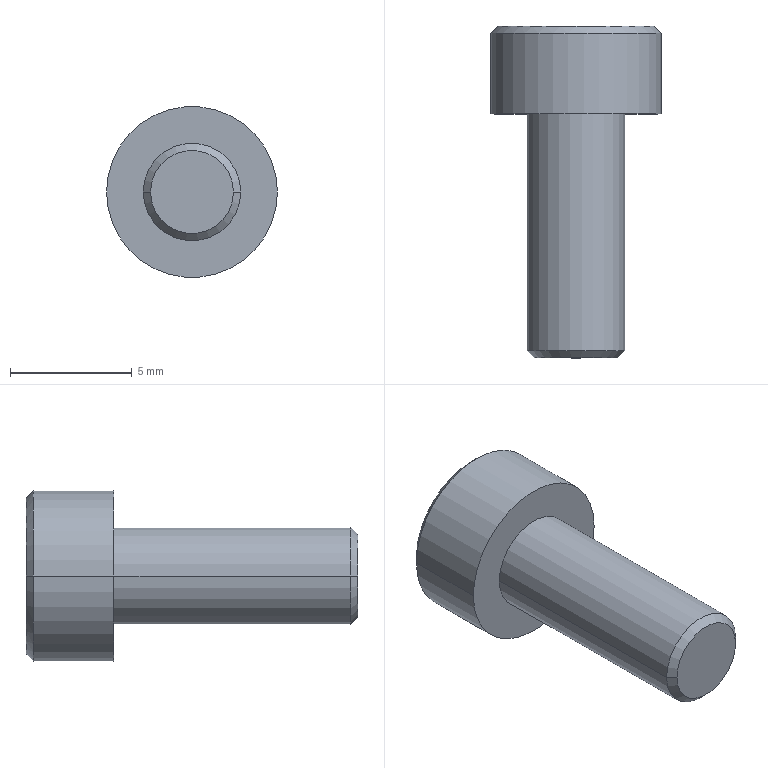Part | NX | 1 solid | 56 faces | box 7 x 13.6 x 7 mm | volume 246.76 mm3 | plane 44 | cone 6 | cylinder 6 | commonest cylinder face diameters 3 x2 4 x2 7 x2
STEP:
#1=CARTESIAN_POINT('',(1.7,-10.,0.));
#2=VERTEX_POINT('',#1);
#3=CARTESIAN_POINT('',(-1.7,-10.,0.));
#4=VERTEX_POINT('',#3);
#5=CARTESIAN_POINT('',(0.,-10.,0.));
#6=DIRECTION('',(0.,1.,0.));
#7=DIRECTION('',(-1.,0.,0.));
#8=AXIS2_PLACEMENT_3D('',#5,#6,#7);
#9=CIRCLE('',#8,1.7);
#10=EDGE_CURVE('',#2,#4,#9,.T.);
#11=ORIENTED_EDGE('',*,*,#10,.F.);
#12=CARTESIAN_POINT('',(0.,-10.,0.));
#13=DIRECTION('',(0.,1.,0.));
#14=DIRECTION('',(-1.,0.,0.));
#15=AXIS2_PLACEMENT_3D('',#12,#13,#14);
#16=CIRCLE('',#15,1.7);
#17=EDGE_CURVE('',#4,#2,#16,.T.);
#18=ORIENTED_EDGE('',*,*,#17,.F.);
#19=EDGE_LOOP('',(#11,#18));
#20=FACE_BOUND('',#19,.T.);
#21=CARTESIAN_POINT('',(0.,-10.,0.));
#22=DIRECTION('',(0.,-1.,0.));
#23=DIRECTION('',(0.,0.,-1.));
#24=AXIS2_PLACEMENT_3D('',#21,#22,#23);
#25=PLANE('',#24);
#26=ADVANCED_FACE('',(#20),#25,.T.);
#27=ORIENTED_EDGE('',*,*,#10,.T.);
#28=CARTESIAN_POINT('',(-2.,-9.7,0.));
#29=VERTEX_POINT('',#28);
#30=CARTESIAN_POINT('',(-1.85,-9.85,0.));
#31=DIRECTION('',(-0.7071,0.7071,0.));
#32=VECTOR('',#31,1000.);
#33=LINE('',#30,#32);
#34=EDGE_CURVE('',#4,#29,#33,.T.);
#35=ORIENTED_EDGE('',*,*,#34,.T.);
#36=CARTESIAN_POINT('',(2.,-9.7,0.));
#37=VERTEX_POINT('',#36);
#38=CARTESIAN_POINT('',(0.,-9.7,0.));
#39=DIRECTION('',(0.,1.,0.));
#40=DIRECTION('',(-1.,0.,0.));
#41=AXIS2_PLACEMENT_3D('',#38,#39,#40);
#42=CIRCLE('',#41,2.);
#43=EDGE_CURVE('',#37,#29,#42,.T.);
#44=ORIENTED_EDGE('',*,*,#43,.F.);
#45=CARTESIAN_POINT('',(1.85,-9.85,0.));
#46=DIRECTION('',(0.7071,0.7071,0.));
#47=VECTOR('',#46,1000.);
#48=LINE('',#45,#47);
#49=EDGE_CURVE('',#2,#37,#48,.T.);
#50=ORIENTED_EDGE('',*,*,#49,.F.);
#51=EDGE_LOOP('',(#27,#35,#44,#50));
#52=FACE_BOUND('',#51,.T.);
#53=CARTESIAN_POINT('',(0.,-9.85,0.));
#54=DIRECTION('',(0.,1.,0.));
#55=DIRECTION('',(1.,0.,0.));
#56=AXIS2_PLACEMENT_3D('',#53,#54,#55);
#57=CONICAL_SURFACE('',#56,1.85,0.7854);
#58=ADVANCED_FACE('',(#52),#57,.T.);
#59=ORIENTED_EDGE('',*,*,#43,.T.);
#60=CARTESIAN_POINT('',(-2.,0.,0.));
#61=VERTEX_POINT('',#60);
#62=CARTESIAN_POINT('',(-2.,4.28,0.));
#63=DIRECTION('',(0.,-1.,0.));
#64=VECTOR('',#63,1000.);
#65=LINE('',#62,#64);
#66=EDGE_CURVE('',#29,#61,#65,.F.);
#67=ORIENTED_EDGE('',*,*,#66,.T.);
#68=CARTESIAN_POINT('',(2.,0.,0.));
#69=VERTEX_POINT('',#68);
#70=CARTESIAN_POINT('',(0.,0.,0.));
#71=DIRECTION('',(0.,-1.,0.));
#72=DIRECTION('',(-1.,0.,0.));
#73=AXIS2_PLACEMENT_3D('',#70,#71,#72);
#74=CIRCLE('',#73,2.);
#75=EDGE_CURVE('',#61,#69,#74,.T.);
#76=ORIENTED_EDGE('',*,*,#75,.T.);
#77=CARTESIAN_POINT('',(2.,4.28,0.));
#78=DIRECTION('',(0.,-1.,0.));
#79=VECTOR('',#78,1000.);
#80=LINE('',#77,#79);
#81=EDGE_CURVE('',#37,#69,#80,.F.);
#82=ORIENTED_EDGE('',*,*,#81,.F.);
#83=EDGE_LOOP('',(#59,#67,#76,#82));
#84=FACE_BOUND('',#83,.T.);
#85=CARTESIAN_POINT('',(0.,4.28,0.));
#86=DIRECTION('',(0.,-1.,0.));
#87=DIRECTION('',(-1.,0.,0.));
#88=AXIS2_PLACEMENT_3D('',#85,#86,#87);
#89=CYLINDRICAL_SURFACE('',#88,2.);
#90=ADVANCED_FACE('',(#84),#89,.T.);
#91=CARTESIAN_POINT('',(0.1875,3.6,1.945));
#92=VERTEX_POINT('',#91);
#93=CARTESIAN_POINT('',(0.4,3.6,1.702));
#94=VERTEX_POINT('',#93);
#95=CARTESIAN_POINT('',(0.1875,3.6,1.945));
#96=DIRECTION('',(0.659,0.,-0.7522));
#97=VECTOR('',#96,1000.);
#98=LINE('',#95,#97);
#99=EDGE_CURVE('',#92,#94,#98,.T.);
#100=ORIENTED_EDGE('',*,*,#99,.T.);
#101=CARTESIAN_POINT('',(0.4,3.55,1.702));
#102=VERTEX_POINT('',#101);
#103=CARTESIAN_POINT('',(0.4,3.55,1.702));
#104=DIRECTION('',(0.,1.,0.));
#105=VECTOR('',#104,1000.);
#106=LINE('',#103,#105);
#107=EDGE_CURVE('',#102,#94,#106,.T.);
#108=ORIENTED_EDGE('',*,*,#107,.F.);
#109=CARTESIAN_POINT('',(0.1875,3.55,1.945));
#110=VERTEX_POINT('',#109);
#111=CARTESIAN_POINT('',(0.4,3.55,1.702));
#112=DIRECTION('',(-0.659,0.,0.7522));
#113=VECTOR('',#112,1000.);
#114=LINE('',#111,#113);
#115=EDGE_CURVE('',#102,#110,#114,.T.);
#116=ORIENTED_EDGE('',*,*,#115,.T.);
#117=CARTESIAN_POINT('',(0.1875,3.55,1.945));
#118=DIRECTION('',(0.,1.,0.));
#119=VECTOR('',#118,1000.);
#120=LINE('',#117,#119);
#121=EDGE_CURVE('',#110,#92,#120,.T.);
#122=ORIENTED_EDGE('',*,*,#121,.T.);
#123=EDGE_LOOP('',(#100,#108,#116,#122));
#124=FACE_BOUND('',#123,.T.);
#125=CARTESIAN_POINT('',(0.1875,3.6,1.945));
#126=DIRECTION('',(0.7522,0.,0.659));
#127=DIRECTION('',(0.,-1.,0.));
#128=AXIS2_PLACEMENT_3D('',#125,#126,#127);
#129=PLANE('',#128);
#130=ADVANCED_FACE('',(#124),#129,.F.);
#131=CARTESIAN_POINT('',(0.1,3.55,1.945));
#132=VERTEX_POINT('',#131);
#133=CARTESIAN_POINT('',(0.4,3.55,1.6));
#134=VERTEX_POINT('',#133);
#135=CARTESIAN_POINT('',(0.1,3.55,1.945));
#136=DIRECTION('',(0.6565,0.,-0.7543));
#137=VECTOR('',#136,1000.);
#138=LINE('',#135,#137);
#139=EDGE_CURVE('',#132,#134,#138,.T.);
#140=ORIENTED_EDGE('',*,*,#139,.F.);
#141=CARTESIAN_POINT('',(0.1,3.55,2.021));
#142=VERTEX_POINT('',#141);
#143=CARTESIAN_POINT('',(0.1,3.55,2.021));
#144=DIRECTION('',(0.,0.,-1.));
#145=VECTOR('',#144,1000.);
#146=LINE('',#143,#145);
#147=EDGE_CURVE('',#142,#132,#146,.T.);
#148=ORIENTED_EDGE('',*,*,#147,.F.);
#149=CARTESIAN_POINT('',(0.4,3.55,2.021));
#150=VERTEX_POINT('',#149);
#151=CARTESIAN_POINT('',(0.4,3.55,2.021));
#152=DIRECTION('',(-1.,0.,0.));
#153=VECTOR('',#152,1000.);
#154=LINE('',#151,#153);
#155=EDGE_CURVE('',#150,#142,#154,.T.);
#156=ORIENTED_EDGE('',*,*,#155,.F.);
#157=CARTESIAN_POINT('',(0.4,3.55,2.2));
#158=VERTEX_POINT('',#157);
#159=CARTESIAN_POINT('',(0.4,3.55,2.2));
#160=DIRECTION('',(0.,0.,-1.));
#161=VECTOR('',#160,1000.);
#162=LINE('',#159,#161);
#163=EDGE_CURVE('',#158,#150,#162,.T.);
#164=ORIENTED_EDGE('',*,*,#163,.F.);
#165=CARTESIAN_POINT('',(0.475,3.55,2.2));
#166=VERTEX_POINT('',#165);
#167=CARTESIAN_POINT('',(0.475,3.55,2.2));
#168=DIRECTION('',(-1.,0.,0.));
#169=VECTOR('',#168,1000.);
#170=LINE('',#167,#169);
#171=EDGE_CURVE('',#166,#158,#170,.T.);
#172=ORIENTED_EDGE('',*,*,#171,.F.);
#173=CARTESIAN_POINT('',(0.475,3.55,2.021));
#174=VERTEX_POINT('',#173);
#175=CARTESIAN_POINT('',(0.475,3.55,2.021));
#176=DIRECTION('',(0.,0.,1.));
#177=VECTOR('',#176,1000.);
#178=LINE('',#175,#177);
#179=EDGE_CURVE('',#174,#166,#178,.T.);
#180=ORIENTED_EDGE('',*,*,#179,.F.);
#181=CARTESIAN_POINT('',(0.6,3.55,2.021));
#182=VERTEX_POINT('',#181);
#183=CARTESIAN_POINT('',(0.6,3.55,2.021));
#184=DIRECTION('',(-1.,0.,0.));
#185=VECTOR('',#184,1000.);
#186=LINE('',#183,#185);
#187=EDGE_CURVE('',#182,#174,#186,.T.);
#188=ORIENTED_EDGE('',*,*,#187,.F.);
#189=CARTESIAN_POINT('',(0.6,3.55,1.945));
#190=VERTEX_POINT('',#189);
#191=CARTESIAN_POINT('',(0.6,3.55,1.945));
#192=DIRECTION('',(0.,0.,1.));
#193=VECTOR('',#192,1000.);
#194=LINE('',#191,#193);
#195=EDGE_CURVE('',#190,#182,#194,.T.);
#196=ORIENTED_EDGE('',*,*,#195,.F.);
#197=CARTESIAN_POINT('',(0.475,3.55,1.945));
#198=VERTEX_POINT('',#197);
#199=CARTESIAN_POINT('',(0.475,3.55,1.945));
#200=DIRECTION('',(1.,0.,0.));
#201=VECTOR('',#200,1000.);
#202=LINE('',#199,#201);
#203=EDGE_CURVE('',#198,#190,#202,.T.);
#204=ORIENTED_EDGE('',*,*,#203,.F.);
#205=CARTESIAN_POINT('',(0.475,3.55,1.6));
#206=VERTEX_POINT('',#205);
#207=CARTESIAN_POINT('',(0.475,3.55,1.6));
#208=DIRECTION('',(0.,0.,1.));
#209=VECTOR('',#208,1000.);
#210=LINE('',#207,#209);
#211=EDGE_CURVE('',#206,#198,#210,.T.);
#212=ORIENTED_EDGE('',*,*,#211,.F.);
#213=CARTESIAN_POINT('',(0.4,3.55,1.6));
#214=DIRECTION('',(1.,0.,0.));
#215=VECTOR('',#214,1000.);
#216=LINE('',#213,#215);
#217=EDGE_CURVE('',#134,#206,#216,.T.);
#218=ORIENTED_EDGE('',*,*,#217,.F.);
#219=EDGE_LOOP('',(#140,#148,#156,#164,#172,#180,#188,#196,#204,#212,#218));
#220=FACE_BOUND('',#219,.T.);
#221=ORIENTED_EDGE('',*,*,#115,.F.);
#222=CARTESIAN_POINT('',(0.4,3.55,1.945));
#223=VERTEX_POINT('',#222);
#224=CARTESIAN_POINT('',(0.4,3.55,1.945));
#225=DIRECTION('',(0.,0.,-1.));
#226=VECTOR('',#225,1000.);
#227=LINE('',#224,#226);
#228=EDGE_CURVE('',#223,#102,#227,.T.);
#229=ORIENTED_EDGE('',*,*,#228,.F.);
#230=CARTESIAN_POINT('',(0.1875,3.55,1.945));
#231=DIRECTION('',(1.,0.,0.));
#232=VECTOR('',#231,1000.);
#233=LINE('',#230,#232);
#234=EDGE_CURVE('',#110,#223,#233,.T.);
#235=ORIENTED_EDGE('',*,*,#234,.F.);
#236=EDGE_LOOP('',(#221,#229,#235));
#237=FACE_BOUND('',#236,.T.);
#238=CARTESIAN_POINT('',(0.,3.55,0.));
#239=DIRECTION('',(0.,1.,0.));
#240=DIRECTION('',(1.,0.,0.));
#241=AXIS2_PLACEMENT_3D('',#238,#239,#240);
#242=PLANE('',#241);
#243=ADVANCED_FACE('',(#220,#237),#242,.T.);
#244=CARTESIAN_POINT('',(-3.5,0.,0.));
#245=VERTEX_POINT('',#244);
#246=CARTESIAN_POINT('',(3.5,0.,0.));
#247=VERTEX_POINT('',#246);
#248=CARTESIAN_POINT('',(0.,0.,0.));
#249=DIRECTION('',(0.,1.,0.));
#250=DIRECTION('',(-1.,0.,0.));
#251=AXIS2_PLACEMENT_3D('',#248,#249,#250);
#252=CIRCLE('',#251,3.5);
#253=EDGE_CURVE('',#245,#247,#252,.T.);
#254=ORIENTED_EDGE('',*,*,#253,.F.);
#255=CARTESIAN_POINT('',(0.,0.,0.));
#256=DIRECTION('',(0.,1.,0.));
#257=DIRECTION('',(-1.,0.,0.));
#258=AXIS2_PLACEMENT_3D('',#255,#256,#257);
#259=CIRCLE('',#258,3.5);
#260=EDGE_CURVE('',#247,#245,#259,.T.);
#261=ORIENTED_EDGE('',*,*,#260,.F.);
#262=EDGE_LOOP('',(#254,#261));
#263=FACE_BOUND('',#262,.T.);
#264=ORIENTED_EDGE('',*,*,#75,.F.);
#265=CARTESIAN_POINT('',(0.,0.,0.));
#266=DIRECTION('',(0.,-1.,0.));
#267=DIRECTION('',(-1.,0.,0.));
#268=AXIS2_PLACEMENT_3D('',#265,#266,#267);
#269=CIRCLE('',#268,2.);
#270=EDGE_CURVE('',#69,#61,#269,.T.);
#271=ORIENTED_EDGE('',*,*,#270,.F.);
#272=EDGE_LOOP('',(#264,#271));
#273=FACE_BOUND('',#272,.T.);
#274=CARTESIAN_POINT('',(0.,0.,0.));
#275=DIRECTION('',(0.,-1.,0.));
#276=DIRECTION('',(0.,0.,-1.));
#277=AXIS2_PLACEMENT_3D('',#274,#275,#276);
#278=PLANE('',#277);
#279=ADVANCED_FACE('',(#263,#273),#278,.T.);
#280=ORIENTED_EDGE('',*,*,#253,.T.);
#281=CARTESIAN_POINT('',(3.5,3.3,0.));
#282=VERTEX_POINT('',#281);
#283=CARTESIAN_POINT('',(3.5,4.28,0.));
#284=DIRECTION('',(0.,-1.,0.));
#285=VECTOR('',#284,1000.);
#286=LINE('',#283,#285);
#287=EDGE_CURVE('',#282,#247,#286,.T.);
#288=ORIENTED_EDGE('',*,*,#287,.F.);
#289=CARTESIAN_POINT('',(-3.5,3.3,0.));
#290=VERTEX_POINT('',#289);
#291=CARTESIAN_POINT('',(0.,3.3,0.));
#292=DIRECTION('',(0.,-1.,0.));
#293=DIRECTION('',(-1.,0.,0.));
#294=AXIS2_PLACEMENT_3D('',#291,#292,#293);
#295=CIRCLE('',#294,3.5);
#296=EDGE_CURVE('',#282,#290,#295,.T.);
#297=ORIENTED_EDGE('',*,*,#296,.T.);
#298=CARTESIAN_POINT('',(-3.5,4.28,0.));
#299=DIRECTION('',(0.,-1.,0.));
#300=VECTOR('',#299,1000.);
#301=LINE('',#298,#300);
#302=EDGE_CURVE('',#290,#245,#301,.T.);
#303=ORIENTED_EDGE('',*,*,#302,.T.);
#304=EDGE_LOOP('',(#280,#288,#297,#303));
#305=FACE_BOUND('',#304,.T.);
#306=CARTESIAN_POINT('',(0.,4.28,0.));
#307=DIRECTION('',(0.,-1.,0.));
#308=DIRECTION('',(-1.,0.,0.));
#309=AXIS2_PLACEMENT_3D('',#306,#307,#308);
#310=CYLINDRICAL_SURFACE('',#309,3.5);
#311=ADVANCED_FACE('',(#305),#310,.T.);
#312=ORIENTED_EDGE('',*,*,#99,.F.);
#313=CARTESIAN_POINT('',(0.4,3.6,1.945));
#314=VERTEX_POINT('',#313);
#315=CARTESIAN_POINT('',(0.1875,3.6,1.945));
#316=DIRECTION('',(1.,0.,0.));
#317=VECTOR('',#316,1000.);
#318=LINE('',#315,#317);
#319=EDGE_CURVE('',#92,#314,#318,.T.);
#320=ORIENTED_EDGE('',*,*,#319,.T.);
#321=CARTESIAN_POINT('',(0.4,3.6,1.945));
#322=DIRECTION('',(0.,0.,-1.));
#323=VECTOR('',#322,1000.);
#324=LINE('',#321,#323);
#325=EDGE_CURVE('',#314,#94,#324,.T.);
#326=ORIENTED_EDGE('',*,*,#325,.T.);
#327=EDGE_LOOP('',(#312,#320,#326));
#328=FACE_BOUND('',#327,.T.);
#329=CARTESIAN_POINT('',(0.,3.6,0.));
#330=DIRECTION('',(0.,-1.,0.));
#331=DIRECTION('',(0.,0.,-1.));
#332=AXIS2_PLACEMENT_3D('',#329,#330,#331);
#333=PLANE('',#332);
#334=ADVANCED_FACE('',(#328),#333,.F.);
#335=CARTESIAN_POINT('',(0.,3.3,0.));
#336=DIRECTION('',(0.,-1.,0.));
#337=DIRECTION('',(-1.,0.,0.));
#338=AXIS2_PLACEMENT_3D('',#335,#336,#337);
#339=CIRCLE('',#338,3.5);
#340=EDGE_CURVE('',#290,#282,#339,.T.);
#341=ORIENTED_EDGE('',*,*,#340,.F.);
#342=CARTESIAN_POINT('',(-3.2,3.6,0.));
#343=VERTEX_POINT('',#342);
#344=CARTESIAN_POINT('',(-3.35,3.45,0.));
#345=DIRECTION('',(-0.7071,-0.7071,0.));
#346=VECTOR('',#345,1000.);
#347=LINE('',#344,#346);
#348=EDGE_CURVE('',#290,#343,#347,.F.);
#349=ORIENTED_EDGE('',*,*,#348,.T.);
#350=CARTESIAN_POINT('',(3.2,3.6,0.));
#351=VERTEX_POINT('',#350);
#352=CARTESIAN_POINT('',(0.,3.6,0.));
#353=DIRECTION('',(0.,-1.,0.));
#354=DIRECTION('',(-1.,0.,0.));
#355=AXIS2_PLACEMENT_3D('',#352,#353,#354);
#356=CIRCLE('',#355,3.2);
#357=EDGE_CURVE('',#343,#351,#356,.T.);
#358=ORIENTED_EDGE('',*,*,#357,.T.);
#359=CARTESIAN_POINT('',(3.35,3.45,0.));
#360=DIRECTION('',(0.7071,-0.7071,0.));
#361=VECTOR('',#360,1000.);
#362=LINE('',#359,#361);
#363=EDGE_CURVE('',#282,#351,#362,.F.);
#364=ORIENTED_EDGE('',*,*,#363,.F.);
#365=EDGE_LOOP('',(#341,#349,#358,#364));
#366=FACE_BOUND('',#365,.T.);
#367=CARTESIAN_POINT('',(0.,3.45,0.));
#368=DIRECTION('',(0.,-1.,0.));
#369=DIRECTION('',(-1.,0.,0.));
#370=AXIS2_PLACEMENT_3D('',#367,#368,#369);
#371=CONICAL_SURFACE('',#370,3.35,0.7854);
#372=ADVANCED_FACE('',(#366),#371,.T.);
#373=ORIENTED_EDGE('',*,*,#357,.F.);
#374=CARTESIAN_POINT('',(0.,3.6,0.));
#375=DIRECTION('',(0.,-1.,0.));
#376=DIRECTION('',(-1.,0.,0.));
#377=AXIS2_PLACEMENT_3D('',#374,#375,#376);
#378=CIRCLE('',#377,3.2);
#379=EDGE_CURVE('',#351,#343,#378,.T.);
#380=ORIENTED_EDGE('',*,*,#379,.F.);
#381=EDGE_LOOP('',(#373,#380));
#382=FACE_BOUND('',#381,.T.);
#383=CARTESIAN_POINT('',(-0.075,3.6,2.2));
#384=VERTEX_POINT('',#383);
#385=CARTESIAN_POINT('',(-0.075,3.6,1.728));
#386=VERTEX_POINT('',#385);
#387=CARTESIAN_POINT('',(-0.075,3.6,2.2));
#388=DIRECTION('',(0.,0.,-1.));
#389=VECTOR('',#388,1000.);
#390=LINE('',#387,#389);
#391=EDGE_CURVE('',#384,#386,#390,.T.);
#392=ORIENTED_EDGE('',*,*,#391,.T.);
#393=CARTESIAN_POINT('',(-0.25,3.6,2.2));
#394=VERTEX_POINT('',#393);
#395=CARTESIAN_POINT('',(-0.25,3.6,2.2));
#396=DIRECTION('',(0.3474,0.,-0.9377));
#397=VECTOR('',#396,1000.);
#398=LINE('',#395,#397);
#399=EDGE_CURVE('',#394,#386,#398,.T.);
#400=ORIENTED_EDGE('',*,*,#399,.F.);
#401=CARTESIAN_POINT('',(-0.35,3.6,2.2));
#402=VERTEX_POINT('',#401);
#403=CARTESIAN_POINT('',(-0.25,3.6,2.2));
#404=DIRECTION('',(-1.,0.,0.));
#405=VECTOR('',#404,1000.);
#406=LINE('',#403,#405);
#407=EDGE_CURVE('',#394,#402,#406,.T.);
#408=ORIENTED_EDGE('',*,*,#407,.T.);
#409=CARTESIAN_POINT('',(-0.525,3.6,1.728));
#410=VERTEX_POINT('',#409);
#411=CARTESIAN_POINT('',(-0.525,3.6,1.728));
#412=DIRECTION('',(0.3474,0.,0.9377));
#413=VECTOR('',#412,1000.);
#414=LINE('',#411,#413);
#415=EDGE_CURVE('',#410,#402,#414,.T.);
#416=ORIENTED_EDGE('',*,*,#415,.F.);
#417=CARTESIAN_POINT('',(-0.525,3.6,2.2));
#418=VERTEX_POINT('',#417);
#419=CARTESIAN_POINT('',(-0.525,3.6,1.728));
#420=DIRECTION('',(0.,0.,1.));
#421=VECTOR('',#420,1000.);
#422=LINE('',#419,#421);
#423=EDGE_CURVE('',#410,#418,#422,.T.);
#424=ORIENTED_EDGE('',*,*,#423,.T.);
#425=CARTESIAN_POINT('',(-0.6,3.6,2.2));
#426=VERTEX_POINT('',#425);
#427=CARTESIAN_POINT('',(-0.525,3.6,2.2));
#428=DIRECTION('',(-1.,0.,0.));
#429=VECTOR('',#428,1000.);
#430=LINE('',#427,#429);
#431=EDGE_CURVE('',#418,#426,#430,.T.);
#432=ORIENTED_EDGE('',*,*,#431,.T.);
#433=CARTESIAN_POINT('',(-0.6,3.6,1.6));
#434=VERTEX_POINT('',#433);
#435=CARTESIAN_POINT('',(-0.6,3.6,2.2));
#436=DIRECTION('',(0.,0.,-1.));
#437=VECTOR('',#436,1000.);
#438=LINE('',#435,#437);
#439=EDGE_CURVE('',#426,#434,#438,.T.);
#440=ORIENTED_EDGE('',*,*,#439,.T.);
#441=CARTESIAN_POINT('',(-0.4875,3.6,1.6));
#442=VERTEX_POINT('',#441);
#443=CARTESIAN_POINT('',(-0.6,3.6,1.6));
#444=DIRECTION('',(1.,0.,0.));
#445=VECTOR('',#444,1000.);
#446=LINE('',#443,#445);
#447=EDGE_CURVE('',#434,#442,#446,.T.);
#448=ORIENTED_EDGE('',*,*,#447,.T.);
#449=CARTESIAN_POINT('',(-0.3,3.6,2.136));
#450=VERTEX_POINT('',#449);
#451=CARTESIAN_POINT('',(-0.3,3.6,2.136));
#452=DIRECTION('',(-0.3301,0.,-0.9439));
#453=VECTOR('',#452,1000.);
#454=LINE('',#451,#453);
#455=EDGE_CURVE('',#450,#442,#454,.T.);
#456=ORIENTED_EDGE('',*,*,#455,.F.);
#457=CARTESIAN_POINT('',(-0.132,3.6,1.656));
#458=VERTEX_POINT('',#457);
#459=CARTESIAN_POINT('',(-0.132,3.6,1.656));
#460=DIRECTION('',(-0.3301,0.,0.9439));
#461=VECTOR('',#460,1000.);
#462=LINE('',#459,#461);
#463=EDGE_CURVE('',#458,#450,#462,.T.);
#464=ORIENTED_EDGE('',*,*,#463,.F.);
#465=CARTESIAN_POINT('',(-1.5,3.6,0.866));
#466=VERTEX_POINT('',#465);
#467=CARTESIAN_POINT('',(-1.5,3.6,0.866));
#468=DIRECTION('',(0.866,0.,0.5));
#469=VECTOR('',#468,1000.);
#470=LINE('',#467,#469);
#471=EDGE_CURVE('',#466,#458,#470,.T.);
#472=ORIENTED_EDGE('',*,*,#471,.F.);
#473=CARTESIAN_POINT('',(-1.5,3.6,-0.866));
#474=VERTEX_POINT('',#473);
#475=CARTESIAN_POINT('',(-1.5,3.6,0.866));
#476=DIRECTION('',(0.,0.,-1.));
#477=VECTOR('',#476,1000.);
#478=LINE('',#475,#477);
#479=EDGE_CURVE('',#466,#474,#478,.T.);
#480=ORIENTED_EDGE('',*,*,#479,.T.);
#481=CARTESIAN_POINT('',(0.,3.6,-1.732));
#482=VERTEX_POINT('',#481);
#483=CARTESIAN_POINT('',(0.,3.6,-1.732));
#484=DIRECTION('',(-0.866,0.,0.5));
#485=VECTOR('',#484,1000.);
#486=LINE('',#483,#485);
#487=EDGE_CURVE('',#482,#474,#486,.T.);
#488=ORIENTED_EDGE('',*,*,#487,.F.);
#489=CARTESIAN_POINT('',(1.5,3.6,-0.866));
#490=VERTEX_POINT('',#489);
#491=CARTESIAN_POINT('',(1.5,3.6,-0.866));
#492=DIRECTION('',(-0.866,0.,-0.5));
#493=VECTOR('',#492,1000.);
#494=LINE('',#491,#493);
#495=EDGE_CURVE('',#490,#482,#494,.T.);
#496=ORIENTED_EDGE('',*,*,#495,.F.);
#497=CARTESIAN_POINT('',(1.5,3.6,0.866));
#498=VERTEX_POINT('',#497);
#499=CARTESIAN_POINT('',(1.5,3.6,-0.866));
#500=DIRECTION('',(0.,0.,1.));
#501=VECTOR('',#500,1000.);
#502=LINE('',#499,#501);
#503=EDGE_CURVE('',#490,#498,#502,.T.);
#504=ORIENTED_EDGE('',*,*,#503,.T.);
#505=CARTESIAN_POINT('',(0.,3.6,1.732));
#506=VERTEX_POINT('',#505);
#507=CARTESIAN_POINT('',(0.,3.6,1.732));
#508=DIRECTION('',(0.866,0.,-0.5));
#509=VECTOR('',#508,1000.);
#510=LINE('',#507,#509);
#511=EDGE_CURVE('',#506,#498,#510,.T.);
#512=ORIENTED_EDGE('',*,*,#511,.F.);
#513=CARTESIAN_POINT('',(0.,3.6,2.2));
#514=VERTEX_POINT('',#513);
#515=CARTESIAN_POINT('',(0.,3.6,1.732));
#516=DIRECTION('',(0.,0.,1.));
#517=VECTOR('',#516,1000.);
#518=LINE('',#515,#517);
#519=EDGE_CURVE('',#506,#514,#518,.T.);
#520=ORIENTED_EDGE('',*,*,#519,.T.);
#521=CARTESIAN_POINT('',(0.,3.6,2.2));
#522=DIRECTION('',(-1.,0.,0.));
#523=VECTOR('',#522,1000.);
#524=LINE('',#521,#523);
#525=EDGE_CURVE('',#514,#384,#524,.T.);
#526=ORIENTED_EDGE('',*,*,#525,.T.);
#527=EDGE_LOOP('',(#392,#400,#408,#416,#424,#432,#440,#448,#456,#464,#472,#480,#488,#496,#504,#512,#520,#526));
#528=FACE_BOUND('',#527,.T.);
#529=CARTESIAN_POINT('',(0.4,3.6,1.6));
#530=VERTEX_POINT('',#529);
#531=CARTESIAN_POINT('',(0.1,3.6,1.945));
#532=VERTEX_POINT('',#531);
#533=CARTESIAN_POINT('',(0.4,3.6,1.6));
#534=DIRECTION('',(-0.6565,0.,0.7543));
#535=VECTOR('',#534,1000.);
#536=LINE('',#533,#535);
#537=EDGE_CURVE('',#530,#532,#536,.T.);
#538=ORIENTED_EDGE('',*,*,#537,.F.);
#539=CARTESIAN_POINT('',(0.475,3.6,1.6));
#540=VERTEX_POINT('',#539);
#541=CARTESIAN_POINT('',(0.4,3.6,1.6));
#542=DIRECTION('',(1.,0.,0.));
#543=VECTOR('',#542,1000.);
#544=LINE('',#541,#543);
#545=EDGE_CURVE('',#530,#540,#544,.T.);
#546=ORIENTED_EDGE('',*,*,#545,.T.);
#547=CARTESIAN_POINT('',(0.475,3.6,1.945));
#548=VERTEX_POINT('',#547);
#549=CARTESIAN_POINT('',(0.475,3.6,1.6));
#550=DIRECTION('',(0.,0.,1.));
#551=VECTOR('',#550,1000.);
#552=LINE('',#549,#551);
#553=EDGE_CURVE('',#540,#548,#552,.T.);
#554=ORIENTED_EDGE('',*,*,#553,.T.);
#555=CARTESIAN_POINT('',(0.6,3.6,1.945));
#556=VERTEX_POINT('',#555);
#557=CARTESIAN_POINT('',(0.475,3.6,1.945));
#558=DIRECTION('',(1.,0.,0.));
#559=VECTOR('',#558,1000.);
#560=LINE('',#557,#559);
#561=EDGE_CURVE('',#548,#556,#560,.T.);
#562=ORIENTED_EDGE('',*,*,#561,.T.);
#563=CARTESIAN_POINT('',(0.6,3.6,2.021));
#564=VERTEX_POINT('',#563);
#565=CARTESIAN_POINT('',(0.6,3.6,1.945));
#566=DIRECTION('',(0.,0.,1.));
#567=VECTOR('',#566,1000.);
#568=LINE('',#565,#567);
#569=EDGE_CURVE('',#556,#564,#568,.T.);
#570=ORIENTED_EDGE('',*,*,#569,.T.);
#571=CARTESIAN_POINT('',(0.475,3.6,2.021));
#572=VERTEX_POINT('',#571);
#573=CARTESIAN_POINT('',(0.6,3.6,2.021));
#574=DIRECTION('',(-1.,0.,0.));
#575=VECTOR('',#574,1000.);
#576=LINE('',#573,#575);
#577=EDGE_CURVE('',#564,#572,#576,.T.);
#578=ORIENTED_EDGE('',*,*,#577,.T.);
#579=CARTESIAN_POINT('',(0.475,3.6,2.2));
#580=VERTEX_POINT('',#579);
#581=CARTESIAN_POINT('',(0.475,3.6,2.021));
#582=DIRECTION('',(0.,0.,1.));
#583=VECTOR('',#582,1000.);
#584=LINE('',#581,#583);
#585=EDGE_CURVE('',#572,#580,#584,.T.);
#586=ORIENTED_EDGE('',*,*,#585,.T.);
#587=CARTESIAN_POINT('',(0.4,3.6,2.2));
#588=VERTEX_POINT('',#587);
#589=CARTESIAN_POINT('',(0.475,3.6,2.2));
#590=DIRECTION('',(-1.,0.,0.));
#591=VECTOR('',#590,1000.);
#592=LINE('',#589,#591);
#593=EDGE_CURVE('',#580,#588,#592,.T.);
#594=ORIENTED_EDGE('',*,*,#593,.T.);
#595=CARTESIAN_POINT('',(0.4,3.6,2.021));
#596=VERTEX_POINT('',#595);
#597=CARTESIAN_POINT('',(0.4,3.6,2.2));
#598=DIRECTION('',(0.,0.,-1.));
#599=VECTOR('',#598,1000.);
#600=LINE('',#597,#599);
#601=EDGE_CURVE('',#588,#596,#600,.T.);
#602=ORIENTED_EDGE('',*,*,#601,.T.);
#603=CARTESIAN_POINT('',(0.1,3.6,2.021));
#604=VERTEX_POINT('',#603);
#605=CARTESIAN_POINT('',(0.4,3.6,2.021));
#606=DIRECTION('',(-1.,0.,0.));
#607=VECTOR('',#606,1000.);
#608=LINE('',#605,#607);
#609=EDGE_CURVE('',#596,#604,#608,.T.);
#610=ORIENTED_EDGE('',*,*,#609,.T.);
#611=CARTESIAN_POINT('',(0.1,3.6,2.021));
#612=DIRECTION('',(0.,0.,-1.));
#613=VECTOR('',#612,1000.);
#614=LINE('',#611,#613);
#615=EDGE_CURVE('',#604,#532,#614,.T.);
#616=ORIENTED_EDGE('',*,*,#615,.T.);
#617=EDGE_LOOP('',(#538,#546,#554,#562,#570,#578,#586,#594,#602,#610,#616));
#618=FACE_BOUND('',#617,.T.);
#619=CARTESIAN_POINT('',(0.,3.6,0.));
#620=DIRECTION('',(0.,-1.,0.));
#621=DIRECTION('',(0.,0.,-1.));
#622=AXIS2_PLACEMENT_3D('',#619,#620,#621);
#623=PLANE('',#622);
#624=ADVANCED_FACE('',(#382,#528,#618),#623,.F.);
#625=ORIENTED_EDGE('',*,*,#319,.F.);
#626=ORIENTED_EDGE('',*,*,#121,.F.);
#627=ORIENTED_EDGE('',*,*,#234,.T.);
#628=CARTESIAN_POINT('',(0.4,3.55,1.945));
#629=DIRECTION('',(0.,1.,0.));
#630=VECTOR('',#629,1000.);
#631=LINE('',#628,#630);
#632=EDGE_CURVE('',#223,#314,#631,.T.);
#633=ORIENTED_EDGE('',*,*,#632,.T.);
#634=EDGE_LOOP('',(#625,#626,#627,#633));
#635=FACE_BOUND('',#634,.T.);
#636=CARTESIAN_POINT('',(0.4,3.6,1.945));
#637=DIRECTION('',(0.,0.,-1.));
#638=DIRECTION('',(0.,-1.,0.));
#639=AXIS2_PLACEMENT_3D('',#636,#637,#638);
#640=PLANE('',#639);
#641=ADVANCED_FACE('',(#635),#640,.F.);
#642=ORIENTED_EDGE('',*,*,#391,.F.);
#643=CARTESIAN_POINT('',(-0.075,3.55,2.2));
#644=VERTEX_POINT('',#643);
#645=CARTESIAN_POINT('',(-0.075,3.55,2.2));
#646=DIRECTION('',(0.,1.,0.));
#647=VECTOR('',#646,1000.);
#648=LINE('',#645,#647);
#649=EDGE_CURVE('',#644,#384,#648,.T.);
#650=ORIENTED_EDGE('',*,*,#649,.F.);
#651=CARTESIAN_POINT('',(-0.075,3.55,1.728));
#652=VERTEX_POINT('',#651);
#653=CARTESIAN_POINT('',(-0.075,3.55,2.2));
#654=DIRECTION('',(0.,0.,-1.));
#655=VECTOR('',#654,1000.);
#656=LINE('',#653,#655);
#657=EDGE_CURVE('',#644,#652,#656,.T.);
#658=ORIENTED_EDGE('',*,*,#657,.T.);
#659=CARTESIAN_POINT('',(-0.075,3.55,1.728));
#660=DIRECTION('',(0.,1.,0.));
#661=VECTOR('',#660,1000.);
#662=LINE('',#659,#661);
#663=EDGE_CURVE('',#652,#386,#662,.T.);
#664=ORIENTED_EDGE('',*,*,#663,.T.);
#665=EDGE_LOOP('',(#642,#650,#658,#664));
#666=FACE_BOUND('',#665,.T.);
#667=CARTESIAN_POINT('',(-0.075,3.6,1.728));
#668=DIRECTION('',(-1.,0.,0.));
#669=DIRECTION('',(0.,0.,1.));
#670=AXIS2_PLACEMENT_3D('',#667,#668,#669);
#671=PLANE('',#670);
#672=ADVANCED_FACE('',(#666),#671,.F.);
#673=ORIENTED_EDGE('',*,*,#399,.T.);
#674=ORIENTED_EDGE('',*,*,#663,.F.);
#675=CARTESIAN_POINT('',(-0.25,3.55,2.2));
#676=VERTEX_POINT('',#675);
#677=CARTESIAN_POINT('',(-0.075,3.55,1.728));
#678=DIRECTION('',(-0.3474,0.,0.9377));
#679=VECTOR('',#678,1000.);
#680=LINE('',#677,#679);
#681=EDGE_CURVE('',#652,#676,#680,.T.);
#682=ORIENTED_EDGE('',*,*,#681,.T.);
#683=CARTESIAN_POINT('',(-0.25,3.55,2.2));
#684=DIRECTION('',(0.,1.,0.));
#685=VECTOR('',#684,1000.);
#686=LINE('',#683,#685);
#687=EDGE_CURVE('',#676,#394,#686,.T.);
#688=ORIENTED_EDGE('',*,*,#687,.T.);
#689=EDGE_LOOP('',(#673,#674,#682,#688));
#690=FACE_BOUND('',#689,.T.);
#691=CARTESIAN_POINT('',(-0.25,3.6,2.2));
#692=DIRECTION('',(0.9377,0.,0.3474));
#693=DIRECTION('',(0.,-1.,0.));
#694=AXIS2_PLACEMENT_3D('',#691,#692,#693);
#695=PLANE('',#694);
#696=ADVANCED_FACE('',(#690),#695,.F.);
#697=ORIENTED_EDGE('',*,*,#407,.F.);
#698=ORIENTED_EDGE('',*,*,#687,.F.);
#699=CARTESIAN_POINT('',(-0.35,3.55,2.2));
#700=VERTEX_POINT('',#699);
#701=CARTESIAN_POINT('',(-0.25,3.55,2.2));
#702=DIRECTION('',(-1.,0.,0.));
#703=VECTOR('',#702,1000.);
#704=LINE('',#701,#703);
#705=EDGE_CURVE('',#676,#700,#704,.T.);
#706=ORIENTED_EDGE('',*,*,#705,.T.);
#707=CARTESIAN_POINT('',(-0.35,3.55,2.2));
#708=DIRECTION('',(0.,1.,0.));
#709=VECTOR('',#708,1000.);
#710=LINE('',#707,#709);
#711=EDGE_CURVE('',#700,#402,#710,.T.);
#712=ORIENTED_EDGE('',*,*,#711,.T.);
#713=EDGE_LOOP('',(#697,#698,#706,#712));
#714=FACE_BOUND('',#713,.T.);
#715=CARTESIAN_POINT('',(-0.35,3.6,2.2));
#716=DIRECTION('',(0.,0.,1.));
#717=DIRECTION('',(1.,0.,0.));
#718=AXIS2_PLACEMENT_3D('',#715,#716,#717);
#719=PLANE('',#718);
#720=ADVANCED_FACE('',(#714),#719,.F.);
#721=ORIENTED_EDGE('',*,*,#415,.T.);
#722=ORIENTED_EDGE('',*,*,#711,.F.);
#723=CARTESIAN_POINT('',(-0.525,3.55,1.728));
#724=VERTEX_POINT('',#723);
#725=CARTESIAN_POINT('',(-0.35,3.55,2.2));
#726=DIRECTION('',(-0.3474,0.,-0.9377));
#727=VECTOR('',#726,1000.);
#728=LINE('',#725,#727);
#729=EDGE_CURVE('',#700,#724,#728,.T.);
#730=ORIENTED_EDGE('',*,*,#729,.T.);
#731=CARTESIAN_POINT('',(-0.525,3.55,1.728));
#732=DIRECTION('',(0.,1.,0.));
#733=VECTOR('',#732,1000.);
#734=LINE('',#731,#733);
#735=EDGE_CURVE('',#724,#410,#734,.T.);
#736=ORIENTED_EDGE('',*,*,#735,.T.);
#737=EDGE_LOOP('',(#721,#722,#730,#736));
#738=FACE_BOUND('',#737,.T.);
#739=CARTESIAN_POINT('',(-0.525,3.6,1.728));
#740=DIRECTION('',(-0.9377,0.,0.3474));
#741=DIRECTION('',(0.,1.,0.));
#742=AXIS2_PLACEMENT_3D('',#739,#740,#741);
#743=PLANE('',#742);
#744=ADVANCED_FACE('',(#738),#743,.F.);
#745=ORIENTED_EDGE('',*,*,#423,.F.);
#746=ORIENTED_EDGE('',*,*,#735,.F.);
#747=CARTESIAN_POINT('',(-0.525,3.55,2.2));
#748=VERTEX_POINT('',#747);
#749=CARTESIAN_POINT('',(-0.525,3.55,1.728));
#750=DIRECTION('',(0.,0.,1.));
#751=VECTOR('',#750,1000.);
#752=LINE('',#749,#751);
#753=EDGE_CURVE('',#724,#748,#752,.T.);
#754=ORIENTED_EDGE('',*,*,#753,.T.);
#755=CARTESIAN_POINT('',(-0.525,3.55,2.2));
#756=DIRECTION('',(0.,1.,0.));
#757=VECTOR('',#756,1000.);
#758=LINE('',#755,#757);
#759=EDGE_CURVE('',#748,#418,#758,.T.);
#760=ORIENTED_EDGE('',*,*,#759,.T.);
#761=EDGE_LOOP('',(#745,#746,#754,#760));
#762=FACE_BOUND('',#761,.T.);
#763=CARTESIAN_POINT('',(-0.525,3.6,2.2));
#764=DIRECTION('',(1.,0.,0.));
#765=DIRECTION('',(0.,1.,0.));
#766=AXIS2_PLACEMENT_3D('',#763,#764,#765);
#767=PLANE('',#766);
#768=ADVANCED_FACE('',(#762),#767,.F.);
#769=ORIENTED_EDGE('',*,*,#431,.F.);
#770=ORIENTED_EDGE('',*,*,#759,.F.);
#771=CARTESIAN_POINT('',(-0.6,3.55,2.2));
#772=VERTEX_POINT('',#771);
#773=CARTESIAN_POINT('',(-0.525,3.55,2.2));
#774=DIRECTION('',(-1.,0.,0.));
#775=VECTOR('',#774,1000.);
#776=LINE('',#773,#775);
#777=EDGE_CURVE('',#748,#772,#776,.T.);
#778=ORIENTED_EDGE('',*,*,#777,.T.);
#779=CARTESIAN_POINT('',(-0.6,3.55,2.2));
#780=DIRECTION('',(0.,1.,0.));
#781=VECTOR('',#780,1000.);
#782=LINE('',#779,#781);
#783=EDGE_CURVE('',#772,#426,#782,.T.);
#784=ORIENTED_EDGE('',*,*,#783,.T.);
#785=EDGE_LOOP('',(#769,#770,#778,#784));
#786=FACE_BOUND('',#785,.T.);
#787=CARTESIAN_POINT('',(-0.6,3.6,2.2));
#788=DIRECTION('',(0.,0.,1.));
#789=DIRECTION('',(1.,0.,0.));
#790=AXIS2_PLACEMENT_3D('',#787,#788,#789);
#791=PLANE('',#790);
#792=ADVANCED_FACE('',(#786),#791,.F.);
#793=ORIENTED_EDGE('',*,*,#439,.F.);
#794=ORIENTED_EDGE('',*,*,#783,.F.);
#795=CARTESIAN_POINT('',(-0.6,3.55,1.6));
#796=VERTEX_POINT('',#795);
#797=CARTESIAN_POINT('',(-0.6,3.55,2.2));
#798=DIRECTION('',(0.,0.,-1.));
#799=VECTOR('',#798,1000.);
#800=LINE('',#797,#799);
#801=EDGE_CURVE('',#772,#796,#800,.T.);
#802=ORIENTED_EDGE('',*,*,#801,.T.);
#803=CARTESIAN_POINT('',(-0.6,3.55,1.6));
#804=DIRECTION('',(0.,1.,0.));
#805=VECTOR('',#804,1000.);
#806=LINE('',#803,#805);
#807=EDGE_CURVE('',#796,#434,#806,.T.);
#808=ORIENTED_EDGE('',*,*,#807,.T.);
#809=EDGE_LOOP('',(#793,#794,#802,#808));
#810=FACE_BOUND('',#809,.T.);
#811=CARTESIAN_POINT('',(-0.6,3.6,1.6));
#812=DIRECTION('',(-1.,0.,0.));
#813=DIRECTION('',(0.,0.,1.));
#814=AXIS2_PLACEMENT_3D('',#811,#812,#813);
#815=PLANE('',#814);
#816=ADVANCED_FACE('',(#810),#815,.F.);
#817=ORIENTED_EDGE('',*,*,#447,.F.);
#818=ORIENTED_EDGE('',*,*,#807,.F.);
#819=CARTESIAN_POINT('',(-0.4875,3.55,1.6));
#820=VERTEX_POINT('',#819);
#821=CARTESIAN_POINT('',(-0.6,3.55,1.6));
#822=DIRECTION('',(1.,0.,0.));
#823=VECTOR('',#822,1000.);
#824=LINE('',#821,#823);
#825=EDGE_CURVE('',#796,#820,#824,.T.);
#826=ORIENTED_EDGE('',*,*,#825,.T.);
#827=CARTESIAN_POINT('',(-0.4875,3.55,1.6));
#828=DIRECTION('',(0.,1.,0.));
#829=VECTOR('',#828,1000.);
#830=LINE('',#827,#829);
#831=EDGE_CURVE('',#820,#442,#830,.T.);
#832=ORIENTED_EDGE('',*,*,#831,.T.);
#833=EDGE_LOOP('',(#817,#818,#826,#832));
#834=FACE_BOUND('',#833,.T.);
#835=CARTESIAN_POINT('',(-0.4875,3.6,1.6));
#836=DIRECTION('',(0.,0.,-1.));
#837=DIRECTION('',(0.,-1.,0.));
#838=AXIS2_PLACEMENT_3D('',#835,#836,#837);
#839=PLANE('',#838);
#840=ADVANCED_FACE('',(#834),#839,.F.);
#841=ORIENTED_EDGE('',*,*,#455,.T.);
#842=ORIENTED_EDGE('',*,*,#831,.F.);
#843=CARTESIAN_POINT('',(-0.3,3.55,2.136));
#844=VERTEX_POINT('',#843);
#845=CARTESIAN_POINT('',(-0.4875,3.55,1.6));
#846=DIRECTION('',(0.3301,0.,0.9439));
#847=VECTOR('',#846,1000.);
#848=LINE('',#845,#847);
#849=EDGE_CURVE('',#820,#844,#848,.T.);
#850=ORIENTED_EDGE('',*,*,#849,.T.);
#851=CARTESIAN_POINT('',(-0.3,3.55,2.136));
#852=DIRECTION('',(0.,1.,0.));
#853=VECTOR('',#852,1000.);
#854=LINE('',#851,#853);
#855=EDGE_CURVE('',#844,#450,#854,.T.);
#856=ORIENTED_EDGE('',*,*,#855,.T.);
#857=EDGE_LOOP('',(#841,#842,#850,#856));
#858=FACE_BOUND('',#857,.T.);
#859=CARTESIAN_POINT('',(-0.3,3.6,2.136));
#860=DIRECTION('',(0.9439,0.,-0.3301));
#861=DIRECTION('',(0.,-1.,0.));
#862=AXIS2_PLACEMENT_3D('',#859,#860,#861);
#863=PLANE('',#862);
#864=ADVANCED_FACE('',(#858),#863,.F.);
#865=ORIENTED_EDGE('',*,*,#463,.T.);
#866=ORIENTED_EDGE('',*,*,#855,.F.);
#867=CARTESIAN_POINT('',(-0.132,3.55,1.656));
#868=VERTEX_POINT('',#867);
#869=CARTESIAN_POINT('',(-0.3,3.55,2.136));
#870=DIRECTION('',(0.3301,0.,-0.9439));
#871=VECTOR('',#870,1000.);
#872=LINE('',#869,#871);
#873=EDGE_CURVE('',#844,#868,#872,.T.);
#874=ORIENTED_EDGE('',*,*,#873,.T.);
#875=CARTESIAN_POINT('',(-0.132,3.55,1.656));
#876=DIRECTION('',(0.,1.,0.));
#877=VECTOR('',#876,1000.);
#878=LINE('',#875,#877);
#879=EDGE_CURVE('',#868,#458,#878,.T.);
#880=ORIENTED_EDGE('',*,*,#879,.T.);
#881=EDGE_LOOP('',(#865,#866,#874,#880));
#882=FACE_BOUND('',#881,.T.);
#883=CARTESIAN_POINT('',(-0.1125,3.6,1.6));
#884=DIRECTION('',(-0.9439,0.,-0.3301));
#885=DIRECTION('',(-0.3301,0.,0.9439));
#886=AXIS2_PLACEMENT_3D('',#883,#884,#885);
#887=PLANE('',#886);
#888=ADVANCED_FACE('',(#882),#887,.F.);
#889=CARTESIAN_POINT('',(0.,3.55,1.732));
#890=VERTEX_POINT('',#889);
#891=CARTESIAN_POINT('',(-0.132,3.55,1.656));
#892=DIRECTION('',(0.866,0.,0.5));
#893=VECTOR('',#892,1000.);
#894=LINE('',#891,#893);
#895=EDGE_CURVE('',#868,#890,#894,.T.);
#896=ORIENTED_EDGE('',*,*,#895,.T.);
#897=CARTESIAN_POINT('',(0.,2.1,1.732));
#898=VERTEX_POINT('',#897);
#899=CARTESIAN_POINT('',(0.,2.1,1.732));
#900=DIRECTION('',(0.,1.,0.));
#901=VECTOR('',#900,1000.);
#902=LINE('',#899,#901);
#903=EDGE_CURVE('',#898,#890,#902,.T.);
#904=ORIENTED_EDGE('',*,*,#903,.F.);
#905=CARTESIAN_POINT('',(-0.75,2.1,1.299));
#906=VERTEX_POINT('',#905);
#907=CARTESIAN_POINT('',(0.,2.1,1.732));
#908=DIRECTION('',(-0.866,0.,-0.5));
#909=VECTOR('',#908,1000.);
#910=LINE('',#907,#909);
#911=EDGE_CURVE('',#898,#906,#910,.T.);
#912=ORIENTED_EDGE('',*,*,#911,.T.);
#913=CARTESIAN_POINT('',(-1.5,2.1,0.866));
#914=VERTEX_POINT('',#913);
#915=CARTESIAN_POINT('',(-0.75,2.1,1.299));
#916=DIRECTION('',(-0.866,0.,-0.5));
#917=VECTOR('',#916,1000.);
#918=LINE('',#915,#917);
#919=EDGE_CURVE('',#906,#914,#918,.T.);
#920=ORIENTED_EDGE('',*,*,#919,.T.);
#921=CARTESIAN_POINT('',(-1.5,2.1,0.866));
#922=DIRECTION('',(0.,1.,0.));
#923=VECTOR('',#922,1000.);
#924=LINE('',#921,#923);
#925=EDGE_CURVE('',#914,#466,#924,.T.);
#926=ORIENTED_EDGE('',*,*,#925,.T.);
#927=ORIENTED_EDGE('',*,*,#471,.T.);
#928=ORIENTED_EDGE('',*,*,#879,.F.);
#929=EDGE_LOOP('',(#896,#904,#912,#920,#926,#927,#928));
#930=FACE_BOUND('',#929,.T.);
#931=CARTESIAN_POINT('',(-1.5,3.6,0.866));
#932=DIRECTION('',(-0.5,0.,0.866));
#933=DIRECTION('',(0.,1.,0.));
#934=AXIS2_PLACEMENT_3D('',#931,#932,#933);
#935=PLANE('',#934);
#936=ADVANCED_FACE('',(#930),#935,.F.);
#937=ORIENTED_EDGE('',*,*,#895,.F.);
#938=ORIENTED_EDGE('',*,*,#873,.F.);
#939=ORIENTED_EDGE('',*,*,#849,.F.);
#940=ORIENTED_EDGE('',*,*,#825,.F.);
#941=ORIENTED_EDGE('',*,*,#801,.F.);
#942=ORIENTED_EDGE('',*,*,#777,.F.);
#943=ORIENTED_EDGE('',*,*,#753,.F.);
#944=ORIENTED_EDGE('',*,*,#729,.F.);
#945=ORIENTED_EDGE('',*,*,#705,.F.);
#946=ORIENTED_EDGE('',*,*,#681,.F.);
#947=ORIENTED_EDGE('',*,*,#657,.F.);
#948=CARTESIAN_POINT('',(0.,3.55,2.2));
#949=VERTEX_POINT('',#948);
#950=CARTESIAN_POINT('',(0.,3.55,2.2));
#951=DIRECTION('',(-1.,0.,0.));
#952=VECTOR('',#951,1000.);
#953=LINE('',#950,#952);
#954=EDGE_CURVE('',#949,#644,#953,.T.);
#955=ORIENTED_EDGE('',*,*,#954,.F.);
#956=CARTESIAN_POINT('',(0.,3.55,1.732));
#957=DIRECTION('',(0.,0.,1.));
#958=VECTOR('',#957,1000.);
#959=LINE('',#956,#958);
#960=EDGE_CURVE('',#890,#949,#959,.T.);
#961=ORIENTED_EDGE('',*,*,#960,.F.);
#962=EDGE_LOOP('',(#937,#938,#939,#940,#941,#942,#943,#944,#945,#946,#947,#955,#961));
#963=FACE_BOUND('',#962,.T.);
#964=CARTESIAN_POINT('',(0.,3.55,0.));
#965=DIRECTION('',(0.,1.,0.));
#966=DIRECTION('',(1.,0.,0.));
#967=AXIS2_PLACEMENT_3D('',#964,#965,#966);
#968=PLANE('',#967);
#969=ADVANCED_FACE('',(#963),#968,.T.);
#970=ORIENTED_EDGE('',*,*,#519,.F.);
#971=CARTESIAN_POINT('',(0.,3.55,1.732));
#972=DIRECTION('',(0.,1.,0.));
#973=VECTOR('',#972,1000.);
#974=LINE('',#971,#973);
#975=EDGE_CURVE('',#890,#506,#974,.T.);
#976=ORIENTED_EDGE('',*,*,#975,.F.);
#977=ORIENTED_EDGE('',*,*,#960,.T.);
#978=CARTESIAN_POINT('',(0.,3.55,2.2));
#979=DIRECTION('',(0.,1.,0.));
#980=VECTOR('',#979,1000.);
#981=LINE('',#978,#980);
#982=EDGE_CURVE('',#949,#514,#981,.T.);
#983=ORIENTED_EDGE('',*,*,#982,.T.);
#984=EDGE_LOOP('',(#970,#976,#977,#983));
#985=FACE_BOUND('',#984,.T.);
#986=CARTESIAN_POINT('',(0.,3.6,2.2));
#987=DIRECTION('',(1.,0.,0.));
#988=DIRECTION('',(0.,1.,0.));
#989=AXIS2_PLACEMENT_3D('',#986,#987,#988);
#990=PLANE('',#989);
#991=ADVANCED_FACE('',(#985),#990,.F.);
#992=ORIENTED_EDGE('',*,*,#525,.F.);
#993=ORIENTED_EDGE('',*,*,#982,.F.);
#994=ORIENTED_EDGE('',*,*,#954,.T.);
#995=ORIENTED_EDGE('',*,*,#649,.T.);
#996=EDGE_LOOP('',(#992,#993,#994,#995));
#997=FACE_BOUND('',#996,.T.);
#998=CARTESIAN_POINT('',(-0.075,3.6,2.2));
#999=DIRECTION('',(0.,0.,1.));
#1000=DIRECTION('',(1.,0.,0.));
#1001=AXIS2_PLACEMENT_3D('',#998,#999,#1000);
#1002=PLANE('',#1001);
#1003=ADVANCED_FACE('',(#997),#1002,.F.);
#1004=ORIENTED_EDGE('',*,*,#975,.T.);
#1005=ORIENTED_EDGE('',*,*,#511,.T.);
#1006=CARTESIAN_POINT('',(1.5,2.1,0.866));
#1007=VERTEX_POINT('',#1006);
#1008=CARTESIAN_POINT('',(1.5,2.1,0.866));
#1009=DIRECTION('',(0.,1.,0.));
#1010=VECTOR('',#1009,1000.);
#1011=LINE('',#1008,#1010);
#1012=EDGE_CURVE('',#1007,#498,#1011,.T.);
#1013=ORIENTED_EDGE('',*,*,#1012,.F.);
#1014=CARTESIAN_POINT('',(0.75,2.1,1.299));
#1015=VERTEX_POINT('',#1014);
#1016=CARTESIAN_POINT('',(1.5,2.1,0.866));
#1017=DIRECTION('',(-0.866,0.,0.5));
#1018=VECTOR('',#1017,1000.);
#1019=LINE('',#1016,#1018);
#1020=EDGE_CURVE('',#1007,#1015,#1019,.T.);
#1021=ORIENTED_EDGE('',*,*,#1020,.T.);
#1022=CARTESIAN_POINT('',(0.75,2.1,1.299));
#1023=DIRECTION('',(-0.866,0.,0.5));
#1024=VECTOR('',#1023,1000.);
#1025=LINE('',#1022,#1024);
#1026=EDGE_CURVE('',#1015,#898,#1025,.T.);
#1027=ORIENTED_EDGE('',*,*,#1026,.T.);
#1028=ORIENTED_EDGE('',*,*,#903,.T.);
#1029=EDGE_LOOP('',(#1004,#1005,#1013,#1021,#1027,#1028));
#1030=FACE_BOUND('',#1029,.T.);
#1031=CARTESIAN_POINT('',(0.,3.6,1.732));
#1032=DIRECTION('',(0.5,0.,0.866));
#1033=DIRECTION('',(0.,-1.,0.));
#1034=AXIS2_PLACEMENT_3D('',#1031,#1032,#1033);
#1035=PLANE('',#1034);
#1036=ADVANCED_FACE('',(#1030),#1035,.F.);
#1037=ORIENTED_EDGE('',*,*,#911,.F.);
#1038=ORIENTED_EDGE('',*,*,#1026,.F.);
#1039=CARTESIAN_POINT('',(0.,2.1,0.));
#1040=DIRECTION('',(0.,1.,0.));
#1041=DIRECTION('',(-0.5,0.,0.866));
#1042=AXIS2_PLACEMENT_3D('',#1039,#1040,#1041);
#1043=CIRCLE('',#1042,1.5);
#1044=EDGE_CURVE('',#906,#1015,#1043,.T.);
#1045=ORIENTED_EDGE('',*,*,#1044,.F.);
#1046=EDGE_LOOP('',(#1037,#1038,#1045));
#1047=FACE_BOUND('',#1046,.T.);
#1048=CARTESIAN_POINT('',(0.,2.1,0.));
#1049=DIRECTION('',(0.,1.,0.));
#1050=DIRECTION('',(1.,0.,0.));
#1051=AXIS2_PLACEMENT_3D('',#1048,#1049,#1050);
#1052=PLANE('',#1051);
#1053=ADVANCED_FACE('',(#1047),#1052,.T.);
#1054=CARTESIAN_POINT('',(-1.5,1.8,0.));
#1055=VERTEX_POINT('',#1054);
#1056=CARTESIAN_POINT('',(1.5,1.8,0.));
#1057=VERTEX_POINT('',#1056);
#1058=CARTESIAN_POINT('',(0.,1.8,0.));
#1059=DIRECTION('',(0.,-1.,0.));
#1060=DIRECTION('',(-1.,0.,0.));
#1061=AXIS2_PLACEMENT_3D('',#1058,#1059,#1060);
#1062=CIRCLE('',#1061,1.5);
#1063=EDGE_CURVE('',#1055,#1057,#1062,.T.);
#1064=ORIENTED_EDGE('',*,*,#1063,.T.);
#1065=CARTESIAN_POINT('',(1.5,2.1,0.));
#1066=VERTEX_POINT('',#1065);
#1067=CARTESIAN_POINT('',(1.5,4.28,0.));
#1068=DIRECTION('',(0.,-1.,0.));
#1069=VECTOR('',#1068,1000.);
#1070=LINE('',#1067,#1069);
#1071=EDGE_CURVE('',#1057,#1066,#1070,.F.);
#1072=ORIENTED_EDGE('',*,*,#1071,.T.);
#1073=CARTESIAN_POINT('',(0.75,2.1,-1.299));
#1074=VERTEX_POINT('',#1073);
#1075=CARTESIAN_POINT('',(0.,2.1,0.));
#1076=DIRECTION('',(0.,1.,0.));
#1077=DIRECTION('',(1.,0.,0.));
#1078=AXIS2_PLACEMENT_3D('',#1075,#1076,#1077);
#1079=CIRCLE('',#1078,1.5);
#1080=EDGE_CURVE('',#1066,#1074,#1079,.T.);
#1081=ORIENTED_EDGE('',*,*,#1080,.T.);
#1082=CARTESIAN_POINT('',(-0.75,2.1,-1.299));
#1083=VERTEX_POINT('',#1082);
#1084=CARTESIAN_POINT('',(0.,2.1,0.));
#1085=DIRECTION('',(0.,1.,0.));
#1086=DIRECTION('',(0.5,0.,-0.866));
#1087=AXIS2_PLACEMENT_3D('',#1084,#1085,#1086);
#1088=CIRCLE('',#1087,1.5);
#1089=EDGE_CURVE('',#1074,#1083,#1088,.T.);
#1090=ORIENTED_EDGE('',*,*,#1089,.T.);
#1091=CARTESIAN_POINT('',(-1.5,2.1,0.));
#1092=VERTEX_POINT('',#1091);
#1093=CARTESIAN_POINT('',(0.,2.1,0.));
#1094=DIRECTION('',(0.,1.,0.));
#1095=DIRECTION('',(-0.5,0.,-0.866));
#1096=AXIS2_PLACEMENT_3D('',#1093,#1094,#1095);
#1097=CIRCLE('',#1096,1.5);
#1098=EDGE_CURVE('',#1083,#1092,#1097,.T.);
#1099=ORIENTED_EDGE('',*,*,#1098,.T.);
#1100=CARTESIAN_POINT('',(-1.5,4.28,0.));
#1101=DIRECTION('',(0.,-1.,0.));
#1102=VECTOR('',#1101,1000.);
#1103=LINE('',#1100,#1102);
#1104=EDGE_CURVE('',#1055,#1092,#1103,.F.);
#1105=ORIENTED_EDGE('',*,*,#1104,.F.);
#1106=EDGE_LOOP('',(#1064,#1072,#1081,#1090,#1099,#1105));
#1107=FACE_BOUND('',#1106,.T.);
#1108=CARTESIAN_POINT('',(0.,4.28,0.));
#1109=DIRECTION('',(0.,-1.,0.));
#1110=DIRECTION('',(-1.,0.,0.));
#1111=AXIS2_PLACEMENT_3D('',#1108,#1109,#1110);
#1112=CYLINDRICAL_SURFACE('',#1111,1.5);
#1113=ADVANCED_FACE('',(#1107),#1112,.F.);
#1114=CARTESIAN_POINT('',(1.5,2.1,0.));
#1115=DIRECTION('',(0.,0.,1.));
#1116=VECTOR('',#1115,1000.);
#1117=LINE('',#1114,#1116);
#1118=EDGE_CURVE('',#1066,#1007,#1117,.T.);
#1119=ORIENTED_EDGE('',*,*,#1118,.F.);
#1120=CARTESIAN_POINT('',(0.,2.1,0.));
#1121=DIRECTION('',(0.,1.,0.));
#1122=DIRECTION('',(0.5,0.,0.866));
#1123=AXIS2_PLACEMENT_3D('',#1120,#1121,#1122);
#1124=CIRCLE('',#1123,1.5);
#1125=EDGE_CURVE('',#1015,#1066,#1124,.T.);
#1126=ORIENTED_EDGE('',*,*,#1125,.F.);
#1127=ORIENTED_EDGE('',*,*,#1020,.F.);
#1128=EDGE_LOOP('',(#1119,#1126,#1127));
#1129=FACE_BOUND('',#1128,.T.);
#1130=CARTESIAN_POINT('',(0.,2.1,0.));
#1131=DIRECTION('',(0.,1.,0.));
#1132=DIRECTION('',(1.,0.,0.));
#1133=AXIS2_PLACEMENT_3D('',#1130,#1131,#1132);
#1134=PLANE('',#1133);
#1135=ADVANCED_FACE('',(#1129),#1134,.T.);
#1136=ORIENTED_EDGE('',*,*,#503,.F.);
#1137=CARTESIAN_POINT('',(1.5,2.1,-0.866));
#1138=VERTEX_POINT('',#1137);
#1139=CARTESIAN_POINT('',(1.5,2.1,-0.866));
#1140=DIRECTION('',(0.,1.,0.));
#1141=VECTOR('',#1140,1000.);
#1142=LINE('',#1139,#1141);
#1143=EDGE_CURVE('',#1138,#490,#1142,.T.);
#1144=ORIENTED_EDGE('',*,*,#1143,.F.);
#1145=CARTESIAN_POINT('',(1.5,2.1,-0.866));
#1146=DIRECTION('',(0.,0.,1.));
#1147=VECTOR('',#1146,1000.);
#1148=LINE('',#1145,#1147);
#1149=EDGE_CURVE('',#1138,#1066,#1148,.T.);
#1150=ORIENTED_EDGE('',*,*,#1149,.T.);
#1151=ORIENTED_EDGE('',*,*,#1118,.T.);
#1152=ORIENTED_EDGE('',*,*,#1012,.T.);
#1153=EDGE_LOOP('',(#1136,#1144,#1150,#1151,#1152));
#1154=FACE_BOUND('',#1153,.T.);
#1155=CARTESIAN_POINT('',(1.5,3.6,0.866));
#1156=DIRECTION('',(1.,0.,0.));
#1157=DIRECTION('',(0.,1.,0.));
#1158=AXIS2_PLACEMENT_3D('',#1155,#1156,#1157);
#1159=PLANE('',#1158);
#1160=ADVANCED_FACE('',(#1154),#1159,.F.);
#1161=ORIENTED_EDGE('',*,*,#1149,.F.);
#1162=CARTESIAN_POINT('',(0.75,2.1,-1.299));
#1163=DIRECTION('',(0.866,0.,0.5));
#1164=VECTOR('',#1163,1000.);
#1165=LINE('',#1162,#1164);
#1166=EDGE_CURVE('',#1074,#1138,#1165,.T.);
#1167=ORIENTED_EDGE('',*,*,#1166,.F.);
#1168=ORIENTED_EDGE('',*,*,#1080,.F.);
#1169=EDGE_LOOP('',(#1161,#1167,#1168));
#1170=FACE_BOUND('',#1169,.T.);
#1171=CARTESIAN_POINT('',(0.,2.1,0.));
#1172=DIRECTION('',(0.,1.,0.));
#1173=DIRECTION('',(1.,0.,0.));
#1174=AXIS2_PLACEMENT_3D('',#1171,#1172,#1173);
#1175=PLANE('',#1174);
#1176=ADVANCED_FACE('',(#1170),#1175,.T.);
#1177=ORIENTED_EDGE('',*,*,#325,.F.);
#1178=ORIENTED_EDGE('',*,*,#632,.F.);
#1179=ORIENTED_EDGE('',*,*,#228,.T.);
#1180=ORIENTED_EDGE('',*,*,#107,.T.);
#1181=EDGE_LOOP('',(#1177,#1178,#1179,#1180));
#1182=FACE_BOUND('',#1181,.T.);
#1183=CARTESIAN_POINT('',(0.4,3.6,1.702));
#1184=DIRECTION('',(-1.,0.,0.));
#1185=DIRECTION('',(0.,0.,1.));
#1186=AXIS2_PLACEMENT_3D('',#1183,#1184,#1185);
#1187=PLANE('',#1186);
#1188=ADVANCED_FACE('',(#1182),#1187,.F.);
#1189=CARTESIAN_POINT('',(-1.5,2.1,-0.866));
#1190=VERTEX_POINT('',#1189);
#1191=CARTESIAN_POINT('',(-1.5,2.1,-0.866));
#1192=DIRECTION('',(0.866,0.,-0.5));
#1193=VECTOR('',#1192,1000.);
#1194=LINE('',#1191,#1193);
#1195=EDGE_CURVE('',#1190,#1083,#1194,.T.);
#1196=ORIENTED_EDGE('',*,*,#1195,.F.);
#1197=CARTESIAN_POINT('',(-1.5,2.1,0.));
#1198=DIRECTION('',(0.,0.,-1.));
#1199=VECTOR('',#1198,1000.);
#1200=LINE('',#1197,#1199);
#1201=EDGE_CURVE('',#1092,#1190,#1200,.T.);
#1202=ORIENTED_EDGE('',*,*,#1201,.F.);
#1203=ORIENTED_EDGE('',*,*,#1098,.F.);
#1204=EDGE_LOOP('',(#1196,#1202,#1203));
#1205=FACE_BOUND('',#1204,.T.);
#1206=CARTESIAN_POINT('',(0.,2.1,0.));
#1207=DIRECTION('',(0.,1.,0.));
#1208=DIRECTION('',(1.,0.,0.));
#1209=AXIS2_PLACEMENT_3D('',#1206,#1207,#1208);
#1210=PLANE('',#1209);
#1211=ADVANCED_FACE('',(#1205),#1210,.T.);
#1212=ORIENTED_EDGE('',*,*,#487,.T.);
#1213=CARTESIAN_POINT('',(-1.5,2.1,-0.866));
#1214=DIRECTION('',(0.,1.,0.));
#1215=VECTOR('',#1214,1000.);
#1216=LINE('',#1213,#1215);
#1217=EDGE_CURVE('',#1190,#474,#1216,.T.);
#1218=ORIENTED_EDGE('',*,*,#1217,.F.);
#1219=ORIENTED_EDGE('',*,*,#1195,.T.);
#1220=CARTESIAN_POINT('',(0.,2.1,-1.732));
#1221=VERTEX_POINT('',#1220);
#1222=CARTESIAN_POINT('',(-0.75,2.1,-1.299));
#1223=DIRECTION('',(0.866,0.,-0.5));
#1224=VECTOR('',#1223,1000.);
#1225=LINE('',#1222,#1224);
#1226=EDGE_CURVE('',#1083,#1221,#1225,.T.);
#1227=ORIENTED_EDGE('',*,*,#1226,.T.);
#1228=CARTESIAN_POINT('',(0.,2.1,-1.732));
#1229=DIRECTION('',(0.,1.,0.));
#1230=VECTOR('',#1229,1000.);
#1231=LINE('',#1228,#1230);
#1232=EDGE_CURVE('',#1221,#482,#1231,.T.);
#1233=ORIENTED_EDGE('',*,*,#1232,.T.);
#1234=EDGE_LOOP('',(#1212,#1218,#1219,#1227,#1233));
#1235=FACE_BOUND('',#1234,.T.);
#1236=CARTESIAN_POINT('',(0.,3.6,-1.732));
#1237=DIRECTION('',(-0.5,0.,-0.866));
#1238=DIRECTION('',(-0.866,0.,0.5));
#1239=AXIS2_PLACEMENT_3D('',#1236,#1237,#1238);
#1240=PLANE('',#1239);
#1241=ADVANCED_FACE('',(#1235),#1240,.F.);
#1242=ORIENTED_EDGE('',*,*,#495,.T.);
#1243=ORIENTED_EDGE('',*,*,#1232,.F.);
#1244=CARTESIAN_POINT('',(0.,2.1,-1.732));
#1245=DIRECTION('',(0.866,0.,0.5));
#1246=VECTOR('',#1245,1000.);
#1247=LINE('',#1244,#1246);
#1248=EDGE_CURVE('',#1221,#1074,#1247,.T.);
#1249=ORIENTED_EDGE('',*,*,#1248,.T.);
#1250=ORIENTED_EDGE('',*,*,#1166,.T.);
#1251=ORIENTED_EDGE('',*,*,#1143,.T.);
#1252=EDGE_LOOP('',(#1242,#1243,#1249,#1250,#1251));
#1253=FACE_BOUND('',#1252,.T.);
#1254=CARTESIAN_POINT('',(1.5,3.6,-0.866));
#1255=DIRECTION('',(0.5,0.,-0.866));
#1256=DIRECTION('',(0.,-1.,0.));
#1257=AXIS2_PLACEMENT_3D('',#1254,#1255,#1256);
#1258=PLANE('',#1257);
#1259=ADVANCED_FACE('',(#1253),#1258,.F.);
#1260=ORIENTED_EDGE('',*,*,#1248,.F.);
#1261=ORIENTED_EDGE('',*,*,#1226,.F.);
#1262=ORIENTED_EDGE('',*,*,#1089,.F.);
#1263=EDGE_LOOP('',(#1260,#1261,#1262));
#1264=FACE_BOUND('',#1263,.T.);
#1265=CARTESIAN_POINT('',(0.,2.1,0.));
#1266=DIRECTION('',(0.,1.,0.));
#1267=DIRECTION('',(1.,0.,0.));
#1268=AXIS2_PLACEMENT_3D('',#1265,#1266,#1267);
#1269=PLANE('',#1268);
#1270=ADVANCED_FACE('',(#1264),#1269,.T.);
#1271=ORIENTED_EDGE('',*,*,#479,.F.);
#1272=ORIENTED_EDGE('',*,*,#925,.F.);
#1273=CARTESIAN_POINT('',(-1.5,2.1,0.866));
#1274=DIRECTION('',(0.,0.,-1.));
#1275=VECTOR('',#1274,1000.);
#1276=LINE('',#1273,#1275);
#1277=EDGE_CURVE('',#914,#1092,#1276,.T.);
#1278=ORIENTED_EDGE('',*,*,#1277,.T.);
#1279=ORIENTED_EDGE('',*,*,#1201,.T.);
#1280=ORIENTED_EDGE('',*,*,#1217,.T.);
#1281=EDGE_LOOP('',(#1271,#1272,#1278,#1279,#1280));
#1282=FACE_BOUND('',#1281,.T.);
#1283=CARTESIAN_POINT('',(-1.5,3.6,-0.866));
#1284=DIRECTION('',(-1.,0.,0.));
#1285=DIRECTION('',(0.,0.,1.));
#1286=AXIS2_PLACEMENT_3D('',#1283,#1284,#1285);
#1287=PLANE('',#1286);
#1288=ADVANCED_FACE('',(#1282),#1287,.F.);
#1289=ORIENTED_EDGE('',*,*,#1277,.F.);
#1290=ORIENTED_EDGE('',*,*,#919,.F.);
#1291=CARTESIAN_POINT('',(0.,2.1,0.));
#1292=DIRECTION('',(0.,1.,0.));
#1293=DIRECTION('',(-1.,0.,0.));
#1294=AXIS2_PLACEMENT_3D('',#1291,#1292,#1293);
#1295=CIRCLE('',#1294,1.5);
#1296=EDGE_CURVE('',#1092,#906,#1295,.T.);
#1297=ORIENTED_EDGE('',*,*,#1296,.F.);
#1298=EDGE_LOOP('',(#1289,#1290,#1297));
#1299=FACE_BOUND('',#1298,.T.);
#1300=CARTESIAN_POINT('',(0.,2.1,0.));
#1301=DIRECTION('',(0.,1.,0.));
#1302=DIRECTION('',(1.,0.,0.));
#1303=AXIS2_PLACEMENT_3D('',#1300,#1301,#1302);
#1304=PLANE('',#1303);
#1305=ADVANCED_FACE('',(#1299),#1304,.T.);
#1306=ORIENTED_EDGE('',*,*,#1063,.F.);
#1307=CARTESIAN_POINT('',(0.,0.8987,0.));
#1308=VERTEX_POINT('',#1307);
#1309=CARTESIAN_POINT('',(-0.765,1.358,0.));
#1310=DIRECTION('',(-0.8572,0.515,0.));
#1311=VECTOR('',#1310,1000.);
#1312=LINE('',#1309,#1311);
#1313=EDGE_CURVE('',#1055,#1308,#1312,.F.);
#1314=ORIENTED_EDGE('',*,*,#1313,.T.);
#1315=CARTESIAN_POINT('',(0.765,1.358,0.));
#1316=DIRECTION('',(0.8572,0.515,0.));
#1317=VECTOR('',#1316,1000.);
#1318=LINE('',#1315,#1317);
#1319=EDGE_CURVE('',#1057,#1308,#1318,.F.);
#1320=ORIENTED_EDGE('',*,*,#1319,.F.);
#1321=EDGE_LOOP('',(#1306,#1314,#1320));
#1322=FACE_BOUND('',#1321,.T.);
#1323=CARTESIAN_POINT('',(0.,1.358,0.));
#1324=DIRECTION('',(0.,1.,0.));
#1325=DIRECTION('',(1.,0.,0.));
#1326=AXIS2_PLACEMENT_3D('',#1323,#1324,#1325);
#1327=CONICAL_SURFACE('',#1326,0.765,1.03);
#1328=ADVANCED_FACE('',(#1322),#1327,.F.);
#1329=ORIENTED_EDGE('',*,*,#615,.F.);
#1330=CARTESIAN_POINT('',(0.1,3.55,2.021));
#1331=DIRECTION('',(0.,1.,0.));
#1332=VECTOR('',#1331,1000.);
#1333=LINE('',#1330,#1332);
#1334=EDGE_CURVE('',#142,#604,#1333,.T.);
#1335=ORIENTED_EDGE('',*,*,#1334,.F.);
#1336=ORIENTED_EDGE('',*,*,#147,.T.);
#1337=CARTESIAN_POINT('',(0.1,3.55,1.945));
#1338=DIRECTION('',(0.,1.,0.));
#1339=VECTOR('',#1338,1000.);
#1340=LINE('',#1337,#1339);
#1341=EDGE_CURVE('',#132,#532,#1340,.T.);
#1342=ORIENTED_EDGE('',*,*,#1341,.T.);
#1343=EDGE_LOOP('',(#1329,#1335,#1336,#1342));
#1344=FACE_BOUND('',#1343,.T.);
#1345=CARTESIAN_POINT('',(0.1,3.6,1.945));
#1346=DIRECTION('',(-1.,0.,0.));
#1347=DIRECTION('',(0.,0.,1.));
#1348=AXIS2_PLACEMENT_3D('',#1345,#1346,#1347);
#1349=PLANE('',#1348);
#1350=ADVANCED_FACE('',(#1344),#1349,.F.);
#1351=ORIENTED_EDGE('',*,*,#537,.T.);
#1352=ORIENTED_EDGE('',*,*,#1341,.F.);
#1353=ORIENTED_EDGE('',*,*,#139,.T.);
#1354=CARTESIAN_POINT('',(0.4,3.55,1.6));
#1355=DIRECTION('',(0.,1.,0.));
#1356=VECTOR('',#1355,1000.);
#1357=LINE('',#1354,#1356);
#1358=EDGE_CURVE('',#134,#530,#1357,.T.);
#1359=ORIENTED_EDGE('',*,*,#1358,.T.);
#1360=EDGE_LOOP('',(#1351,#1352,#1353,#1359));
#1361=FACE_BOUND('',#1360,.T.);
#1362=CARTESIAN_POINT('',(0.4,3.6,1.6));
#1363=DIRECTION('',(-0.7543,0.,-0.6565));
#1364=DIRECTION('',(-0.6565,0.,0.7543));
#1365=AXIS2_PLACEMENT_3D('',#1362,#1363,#1364);
#1366=PLANE('',#1365);
#1367=ADVANCED_FACE('',(#1361),#1366,.F.);
#1368=ORIENTED_EDGE('',*,*,#545,.F.);
#1369=ORIENTED_EDGE('',*,*,#1358,.F.);
#1370=ORIENTED_EDGE('',*,*,#217,.T.);
#1371=CARTESIAN_POINT('',(0.475,3.55,1.6));
#1372=DIRECTION('',(0.,1.,0.));
#1373=VECTOR('',#1372,1000.);
#1374=LINE('',#1371,#1373);
#1375=EDGE_CURVE('',#206,#540,#1374,.T.);
#1376=ORIENTED_EDGE('',*,*,#1375,.T.);
#1377=EDGE_LOOP('',(#1368,#1369,#1370,#1376));
#1378=FACE_BOUND('',#1377,.T.);
#1379=CARTESIAN_POINT('',(0.475,3.6,1.6));
#1380=DIRECTION('',(0.,0.,-1.));
#1381=DIRECTION('',(0.,-1.,0.));
#1382=AXIS2_PLACEMENT_3D('',#1379,#1380,#1381);
#1383=PLANE('',#1382);
#1384=ADVANCED_FACE('',(#1378),#1383,.F.);
#1385=ORIENTED_EDGE('',*,*,#553,.F.);
#1386=ORIENTED_EDGE('',*,*,#1375,.F.);
#1387=ORIENTED_EDGE('',*,*,#211,.T.);
#1388=CARTESIAN_POINT('',(0.475,3.55,1.945));
#1389=DIRECTION('',(0.,1.,0.));
#1390=VECTOR('',#1389,1000.);
#1391=LINE('',#1388,#1390);
#1392=EDGE_CURVE('',#198,#548,#1391,.T.);
#1393=ORIENTED_EDGE('',*,*,#1392,.T.);
#1394=EDGE_LOOP('',(#1385,#1386,#1387,#1393));
#1395=FACE_BOUND('',#1394,.T.);
#1396=CARTESIAN_POINT('',(0.475,3.6,1.945));
#1397=DIRECTION('',(1.,0.,0.));
#1398=DIRECTION('',(0.,1.,0.));
#1399=AXIS2_PLACEMENT_3D('',#1396,#1397,#1398);
#1400=PLANE('',#1399);
#1401=ADVANCED_FACE('',(#1395),#1400,.F.);
#1402=ORIENTED_EDGE('',*,*,#561,.F.);
#1403=ORIENTED_EDGE('',*,*,#1392,.F.);
#1404=ORIENTED_EDGE('',*,*,#203,.T.);
#1405=CARTESIAN_POINT('',(0.6,3.55,1.945));
#1406=DIRECTION('',(0.,1.,0.));
#1407=VECTOR('',#1406,1000.);
#1408=LINE('',#1405,#1407);
#1409=EDGE_CURVE('',#190,#556,#1408,.T.);
#1410=ORIENTED_EDGE('',*,*,#1409,.T.);
#1411=EDGE_LOOP('',(#1402,#1403,#1404,#1410));
#1412=FACE_BOUND('',#1411,.T.);
#1413=CARTESIAN_POINT('',(0.6,3.6,1.945));
#1414=DIRECTION('',(0.,0.,-1.));
#1415=DIRECTION('',(0.,-1.,0.));
#1416=AXIS2_PLACEMENT_3D('',#1413,#1414,#1415);
#1417=PLANE('',#1416);
#1418=ADVANCED_FACE('',(#1412),#1417,.F.);
#1419=ORIENTED_EDGE('',*,*,#569,.F.);
#1420=ORIENTED_EDGE('',*,*,#1409,.F.);
#1421=ORIENTED_EDGE('',*,*,#195,.T.);
#1422=CARTESIAN_POINT('',(0.6,3.55,2.021));
#1423=DIRECTION('',(0.,1.,0.));
#1424=VECTOR('',#1423,1000.);
#1425=LINE('',#1422,#1424);
#1426=EDGE_CURVE('',#182,#564,#1425,.T.);
#1427=ORIENTED_EDGE('',*,*,#1426,.T.);
#1428=EDGE_LOOP('',(#1419,#1420,#1421,#1427));
#1429=FACE_BOUND('',#1428,.T.);
#1430=CARTESIAN_POINT('',(0.6,3.6,2.021));
#1431=DIRECTION('',(1.,0.,0.));
#1432=DIRECTION('',(0.,1.,0.));
#1433=AXIS2_PLACEMENT_3D('',#1430,#1431,#1432);
#1434=PLANE('',#1433);
#1435=ADVANCED_FACE('',(#1429),#1434,.F.);
#1436=ORIENTED_EDGE('',*,*,#577,.F.);
#1437=ORIENTED_EDGE('',*,*,#1426,.F.);
#1438=ORIENTED_EDGE('',*,*,#187,.T.);
#1439=CARTESIAN_POINT('',(0.475,3.55,2.021));
#1440=DIRECTION('',(0.,1.,0.));
#1441=VECTOR('',#1440,1000.);
#1442=LINE('',#1439,#1441);
#1443=EDGE_CURVE('',#174,#572,#1442,.T.);
#1444=ORIENTED_EDGE('',*,*,#1443,.T.);
#1445=EDGE_LOOP('',(#1436,#1437,#1438,#1444));
#1446=FACE_BOUND('',#1445,.T.);
#1447=CARTESIAN_POINT('',(0.475,3.6,2.021));
#1448=DIRECTION('',(0.,0.,1.));
#1449=DIRECTION('',(1.,0.,0.));
#1450=AXIS2_PLACEMENT_3D('',#1447,#1448,#1449);
#1451=PLANE('',#1450);
#1452=ADVANCED_FACE('',(#1446),#1451,.F.);
#1453=ORIENTED_EDGE('',*,*,#585,.F.);
#1454=ORIENTED_EDGE('',*,*,#1443,.F.);
#1455=ORIENTED_EDGE('',*,*,#179,.T.);
#1456=CARTESIAN_POINT('',(0.475,3.55,2.2));
#1457=DIRECTION('',(0.,1.,0.));
#1458=VECTOR('',#1457,1000.);
#1459=LINE('',#1456,#1458);
#1460=EDGE_CURVE('',#166,#580,#1459,.T.);
#1461=ORIENTED_EDGE('',*,*,#1460,.T.);
#1462=EDGE_LOOP('',(#1453,#1454,#1455,#1461));
#1463=FACE_BOUND('',#1462,.T.);
#1464=CARTESIAN_POINT('',(0.475,3.6,2.2));
#1465=DIRECTION('',(1.,0.,0.));
#1466=DIRECTION('',(0.,1.,0.));
#1467=AXIS2_PLACEMENT_3D('',#1464,#1465,#1466);
#1468=PLANE('',#1467);
#1469=ADVANCED_FACE('',(#1463),#1468,.F.);
#1470=ORIENTED_EDGE('',*,*,#593,.F.);
#1471=ORIENTED_EDGE('',*,*,#1460,.F.);
#1472=ORIENTED_EDGE('',*,*,#171,.T.);
#1473=CARTESIAN_POINT('',(0.4,3.55,2.2));
#1474=DIRECTION('',(0.,1.,0.));
#1475=VECTOR('',#1474,1000.);
#1476=LINE('',#1473,#1475);
#1477=EDGE_CURVE('',#158,#588,#1476,.T.);
#1478=ORIENTED_EDGE('',*,*,#1477,.T.);
#1479=EDGE_LOOP('',(#1470,#1471,#1472,#1478));
#1480=FACE_BOUND('',#1479,.T.);
#1481=CARTESIAN_POINT('',(0.4,3.6,2.2));
#1482=DIRECTION('',(0.,0.,1.));
#1483=DIRECTION('',(1.,0.,0.));
#1484=AXIS2_PLACEMENT_3D('',#1481,#1482,#1483);
#1485=PLANE('',#1484);
#1486=ADVANCED_FACE('',(#1480),#1485,.F.);
#1487=ORIENTED_EDGE('',*,*,#601,.F.);
#1488=ORIENTED_EDGE('',*,*,#1477,.F.);
#1489=ORIENTED_EDGE('',*,*,#163,.T.);
#1490=CARTESIAN_POINT('',(0.4,3.55,2.021));
#1491=DIRECTION('',(0.,1.,0.));
#1492=VECTOR('',#1491,1000.);
#1493=LINE('',#1490,#1492);
#1494=EDGE_CURVE('',#150,#596,#1493,.T.);
#1495=ORIENTED_EDGE('',*,*,#1494,.T.);
#1496=EDGE_LOOP('',(#1487,#1488,#1489,#1495));
#1497=FACE_BOUND('',#1496,.T.);
#1498=CARTESIAN_POINT('',(0.4,3.6,2.021));
#1499=DIRECTION('',(-1.,0.,0.));
#1500=DIRECTION('',(0.,0.,1.));
#1501=AXIS2_PLACEMENT_3D('',#1498,#1499,#1500);
#1502=PLANE('',#1501);
#1503=ADVANCED_FACE('',(#1497),#1502,.F.);
#1504=ORIENTED_EDGE('',*,*,#609,.F.);
#1505=ORIENTED_EDGE('',*,*,#1494,.F.);
#1506=ORIENTED_EDGE('',*,*,#155,.T.);
#1507=ORIENTED_EDGE('',*,*,#1334,.T.);
#1508=EDGE_LOOP('',(#1504,#1505,#1506,#1507));
#1509=FACE_BOUND('',#1508,.T.);
#1510=CARTESIAN_POINT('',(0.1,3.6,2.021));
#1511=DIRECTION('',(0.,0.,1.));
#1512=DIRECTION('',(1.,0.,0.));
#1513=AXIS2_PLACEMENT_3D('',#1510,#1511,#1512);
#1514=PLANE('',#1513);
#1515=ADVANCED_FACE('',(#1509),#1514,.F.);
#1516=ORIENTED_EDGE('',*,*,#340,.T.);
#1517=ORIENTED_EDGE('',*,*,#287,.T.);
#1518=ORIENTED_EDGE('',*,*,#260,.T.);
#1519=ORIENTED_EDGE('',*,*,#302,.F.);
#1520=EDGE_LOOP('',(#1516,#1517,#1518,#1519));
#1521=FACE_BOUND('',#1520,.T.);
#1522=CARTESIAN_POINT('',(0.,4.28,0.));
#1523=DIRECTION('',(0.,-1.,0.));
#1524=DIRECTION('',(-1.,0.,0.));
#1525=AXIS2_PLACEMENT_3D('',#1522,#1523,#1524);
#1526=CYLINDRICAL_SURFACE('',#1525,3.5);
#1527=ADVANCED_FACE('',(#1521),#1526,.T.);
#1528=ORIENTED_EDGE('',*,*,#49,.T.);
#1529=CARTESIAN_POINT('',(0.,-9.7,0.));
#1530=DIRECTION('',(0.,1.,0.));
#1531=DIRECTION('',(-1.,0.,0.));
#1532=AXIS2_PLACEMENT_3D('',#1529,#1530,#1531);
#1533=CIRCLE('',#1532,2.);
#1534=EDGE_CURVE('',#29,#37,#1533,.T.);
#1535=ORIENTED_EDGE('',*,*,#1534,.F.);
#1536=ORIENTED_EDGE('',*,*,#34,.F.);
#1537=ORIENTED_EDGE('',*,*,#17,.T.);
#1538=EDGE_LOOP('',(#1528,#1535,#1536,#1537));
#1539=FACE_BOUND('',#1538,.T.);
#1540=CARTESIAN_POINT('',(0.,-9.85,0.));
#1541=DIRECTION('',(0.,1.,0.));
#1542=DIRECTION('',(1.,0.,0.));
#1543=AXIS2_PLACEMENT_3D('',#1540,#1541,#1542);
#1544=CONICAL_SURFACE('',#1543,1.85,0.7854);
#1545=ADVANCED_FACE('',(#1539),#1544,.T.);
#1546=ORIENTED_EDGE('',*,*,#1104,.T.);
#1547=ORIENTED_EDGE('',*,*,#1296,.T.);
#1548=ORIENTED_EDGE('',*,*,#1044,.T.);
#1549=ORIENTED_EDGE('',*,*,#1125,.T.);
#1550=ORIENTED_EDGE('',*,*,#1071,.F.);
#1551=CARTESIAN_POINT('',(0.,1.8,0.));
#1552=DIRECTION('',(0.,-1.,0.));
#1553=DIRECTION('',(-1.,0.,0.));
#1554=AXIS2_PLACEMENT_3D('',#1551,#1552,#1553);
#1555=CIRCLE('',#1554,1.5);
#1556=EDGE_CURVE('',#1057,#1055,#1555,.T.);
#1557=ORIENTED_EDGE('',*,*,#1556,.T.);
#1558=EDGE_LOOP('',(#1546,#1547,#1548,#1549,#1550,#1557));
#1559=FACE_BOUND('',#1558,.T.);
#1560=CARTESIAN_POINT('',(0.,4.28,0.));
#1561=DIRECTION('',(0.,-1.,0.));
#1562=DIRECTION('',(-1.,0.,0.));
#1563=AXIS2_PLACEMENT_3D('',#1560,#1561,#1562);
#1564=CYLINDRICAL_SURFACE('',#1563,1.5);
#1565=ADVANCED_FACE('',(#1559),#1564,.F.);
#1566=ORIENTED_EDGE('',*,*,#348,.F.);
#1567=ORIENTED_EDGE('',*,*,#296,.F.);
#1568=ORIENTED_EDGE('',*,*,#363,.T.);
#1569=ORIENTED_EDGE('',*,*,#379,.T.);
#1570=EDGE_LOOP('',(#1566,#1567,#1568,#1569));
#1571=FACE_BOUND('',#1570,.T.);
#1572=CARTESIAN_POINT('',(0.,3.45,0.));
#1573=DIRECTION('',(0.,-1.,0.));
#1574=DIRECTION('',(-1.,0.,0.));
#1575=AXIS2_PLACEMENT_3D('',#1572,#1573,#1574);
#1576=CONICAL_SURFACE('',#1575,3.35,0.7854);
#1577=ADVANCED_FACE('',(#1571),#1576,.T.);
#1578=ORIENTED_EDGE('',*,*,#66,.F.);
#1579=ORIENTED_EDGE('',*,*,#1534,.T.);
#1580=ORIENTED_EDGE('',*,*,#81,.T.);
#1581=ORIENTED_EDGE('',*,*,#270,.T.);
#1582=EDGE_LOOP('',(#1578,#1579,#1580,#1581));
#1583=FACE_BOUND('',#1582,.T.);
#1584=CARTESIAN_POINT('',(0.,4.28,0.));
#1585=DIRECTION('',(0.,-1.,0.));
#1586=DIRECTION('',(-1.,0.,0.));
#1587=AXIS2_PLACEMENT_3D('',#1584,#1585,#1586);
#1588=CYLINDRICAL_SURFACE('',#1587,2.);
#1589=ADVANCED_FACE('',(#1583),#1588,.T.);
#1590=ORIENTED_EDGE('',*,*,#1313,.F.);
#1591=ORIENTED_EDGE('',*,*,#1556,.F.);
#1592=ORIENTED_EDGE('',*,*,#1319,.T.);
#1593=EDGE_LOOP('',(#1590,#1591,#1592));
#1594=FACE_BOUND('',#1593,.T.);
#1595=CARTESIAN_POINT('',(0.,1.358,0.));
#1596=DIRECTION('',(0.,1.,0.));
#1597=DIRECTION('',(1.,0.,0.));
#1598=AXIS2_PLACEMENT_3D('',#1595,#1596,#1597);
#1599=CONICAL_SURFACE('',#1598,0.765,1.03);
#1600=ADVANCED_FACE('',(#1594),#1599,.F.);
#1601=CLOSED_SHELL('',(#26,#58,#90,#130,#243,#279,#311,#334,#372,#624,#641,#672,#696,#720,#744,#768,#792,#816,#840,#864,#888,#936,#969,#991,#1003,#1036,#1053,#1113,#1135,#1160,#1176,#1188,#1211,#1241,#1259,#1270,#1288,#1305,#1328,#1350,#1367,#1384,#1401,#1418,#1435,#1452,#1469,#1486,#1503,#1515,#1527,#1545,#1565,#1577,#1589,#1600));
#1602=MANIFOLD_SOLID_BREP('',#1601);
#1603=(LENGTH_UNIT()NAMED_UNIT(*)SI_UNIT(.MILLI.,.METRE.));
#1604=UNCERTAINTY_MEASURE_WITH_UNIT(LENGTH_MEASURE(0.00001),#1603,'','');
#1605=(NAMED_UNIT(*)PLANE_ANGLE_UNIT()SI_UNIT($,.RADIAN.));
#1606=(NAMED_UNIT(*)SI_UNIT($,.STERADIAN.)SOLID_ANGLE_UNIT());
#1607=(GEOMETRIC_REPRESENTATION_CONTEXT(3)GLOBAL_UNCERTAINTY_ASSIGNED_CONTEXT((#1604))GLOBAL_UNIT_ASSIGNED_CONTEXT((#1603,#1605,#1606))REPRESENTATION_CONTEXT('',''));
#1608=ADVANCED_BREP_SHAPE_REPRESENTATION('',(#1602),#1607);